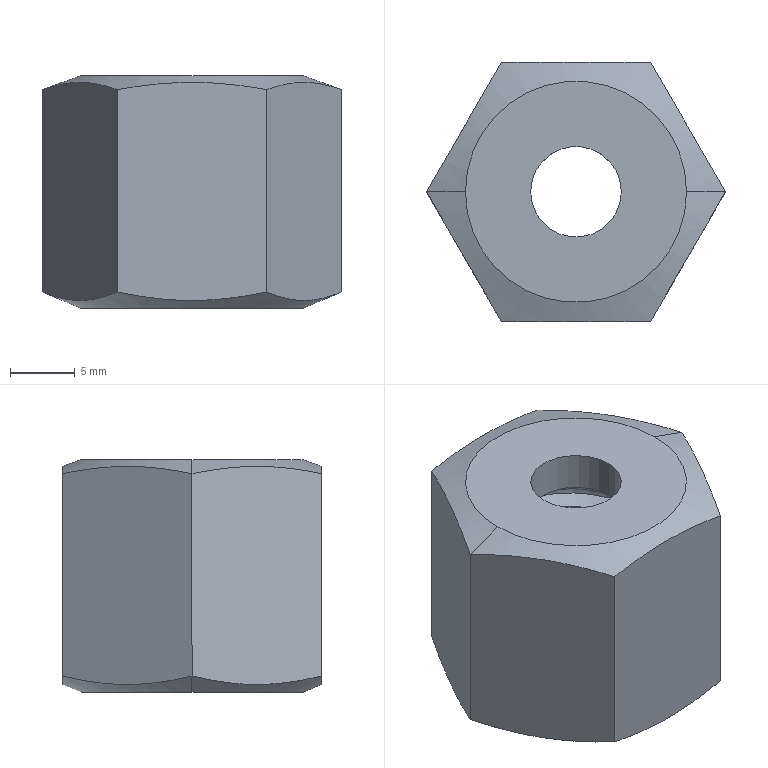Part | SolidWorks | features BaseBody 1 | 1 solid | 52 faces | box 23.094 x 20 x 18 mm | volume 4012 mm3 | cylinder 35 | plane 10 | cone 4 | spline 3 | commonest cylinder face diameters 12 x17 14 x16 7 x2